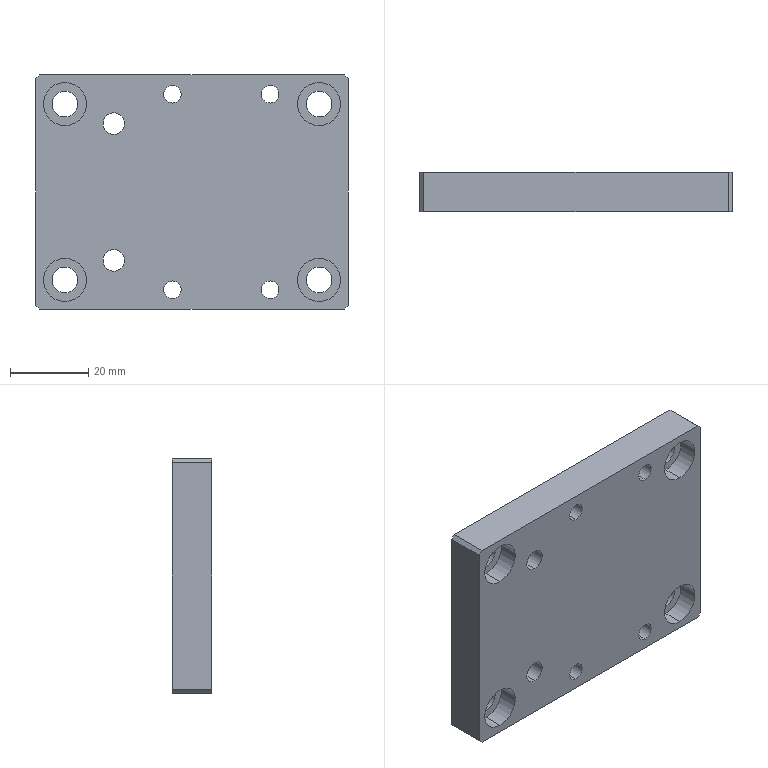Part | SolidWorks | features BaseBody 1 | 1 solid | 60 faces | box 80 x 10 x 60 mm | volume 43027 mm3 | cylinder 40 | plane 20 | commonest cylinder face diameters 4.5 x8 6.6 x8 8 x8 11 x8 5.5 x4 10 x4